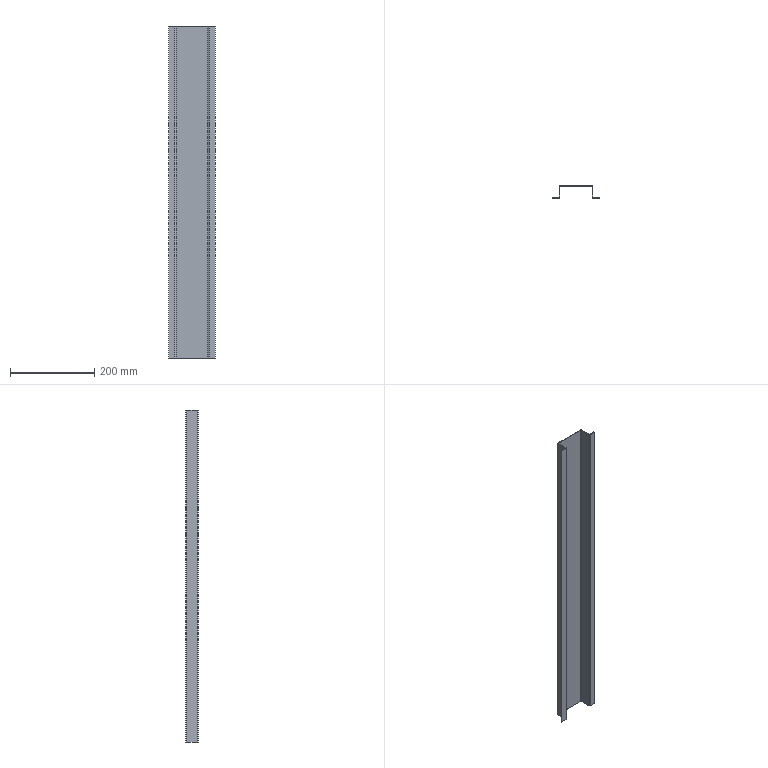Part | SolidWorks | features FlatPattern 1, SMBaseFlange 1, SheetMetal 1 | 1 solid | 38 faces | box 110 x 30 x 790 mm | volume 195352 mm3 | plane 30 | cylinder 8 | commonest cylinder face diameters 1 x4 4 x4
STEP:
#1=CARTESIAN_POINT('',(-40.,0.5,395.));
#2=VERTEX_POINT('',#1);
#3=CARTESIAN_POINT('',(-38.5,0.5,395.));
#4=VERTEX_POINT('',#3);
#5=CARTESIAN_POINT('',(-40.,0.5,395.));
#6=DIRECTION('',(1.,0.,0.));
#7=VECTOR('',#6,1000.);
#8=LINE('',#5,#7);
#9=EDGE_CURVE('',#2,#4,#8,.T.);
#10=ORIENTED_EDGE('',*,*,#9,.F.);
#11=CARTESIAN_POINT('',(-40.5,0.,395.));
#12=VERTEX_POINT('',#11);
#13=CARTESIAN_POINT('',(-40.5,0.5,395.));
#14=DIRECTION('',(0.,0.,-1.));
#15=DIRECTION('',(-1.,0.,0.));
#16=AXIS2_PLACEMENT_3D('',#13,#14,#15);
#17=CIRCLE('',#16,0.5);
#18=EDGE_CURVE('',#2,#12,#17,.T.);
#19=ORIENTED_EDGE('',*,*,#18,.T.);
#20=CARTESIAN_POINT('',(-40.5,-1.5,395.));
#21=VERTEX_POINT('',#20);
#22=CARTESIAN_POINT('',(-40.5,-1.5,395.));
#23=DIRECTION('',(0.,1.,0.));
#24=VECTOR('',#23,1000.);
#25=LINE('',#22,#24);
#26=EDGE_CURVE('',#21,#12,#25,.T.);
#27=ORIENTED_EDGE('',*,*,#26,.F.);
#28=CARTESIAN_POINT('',(-40.5,0.5,395.));
#29=DIRECTION('',(0.,0.,-1.));
#30=DIRECTION('',(1.,0.,0.));
#31=AXIS2_PLACEMENT_3D('',#28,#29,#30);
#32=CIRCLE('',#31,2.);
#33=EDGE_CURVE('',#4,#21,#32,.T.);
#34=ORIENTED_EDGE('',*,*,#33,.F.);
#35=EDGE_LOOP('',(#10,#19,#27,#34));
#36=FACE_OUTER_BOUND('',#35,.T.);
#37=CARTESIAN_POINT('',(-40.,0.5,395.));
#38=DIRECTION('',(0.,0.,1.));
#39=DIRECTION('',(1.,0.,0.));
#40=AXIS2_PLACEMENT_3D('',#37,#38,#39);
#41=PLANE('',#40);
#42=ADVANCED_FACE('',(#36),#41,.T.);
#43=CARTESIAN_POINT('',(-40.,26.5,395.));
#44=VERTEX_POINT('',#43);
#45=CARTESIAN_POINT('',(-40.,0.,395.));
#46=DIRECTION('',(0.,-1.,0.));
#47=VECTOR('',#46,1000.);
#48=LINE('',#45,#47);
#49=EDGE_CURVE('',#44,#2,#48,.T.);
#50=ORIENTED_EDGE('',*,*,#49,.T.);
#51=ORIENTED_EDGE('',*,*,#9,.T.);
#52=CARTESIAN_POINT('',(-38.5,26.5,395.));
#53=VERTEX_POINT('',#52);
#54=CARTESIAN_POINT('',(-38.5,0.,395.));
#55=DIRECTION('',(0.,-1.,0.));
#56=VECTOR('',#55,1000.);
#57=LINE('',#54,#56);
#58=EDGE_CURVE('',#53,#4,#57,.T.);
#59=ORIENTED_EDGE('',*,*,#58,.F.);
#60=CARTESIAN_POINT('',(-38.5,26.5,395.));
#61=DIRECTION('',(-1.,0.,0.));
#62=VECTOR('',#61,1000.);
#63=LINE('',#60,#62);
#64=EDGE_CURVE('',#53,#44,#63,.T.);
#65=ORIENTED_EDGE('',*,*,#64,.T.);
#66=EDGE_LOOP('',(#50,#51,#59,#65));
#67=FACE_OUTER_BOUND('',#66,.T.);
#68=CARTESIAN_POINT('',(-40.5,-1.5,395.));
#69=DIRECTION('',(0.,0.,1.));
#70=DIRECTION('',(1.,0.,0.));
#71=AXIS2_PLACEMENT_3D('',#68,#69,#70);
#72=PLANE('',#71);
#73=ADVANCED_FACE('',(#67),#72,.T.);
#74=CARTESIAN_POINT('',(-40.5,0.,-395.));
#75=VERTEX_POINT('',#74);
#76=CARTESIAN_POINT('',(-40.5,-1.5,-395.));
#77=VERTEX_POINT('',#76);
#78=CARTESIAN_POINT('',(-40.5,0.,-395.));
#79=DIRECTION('',(0.,-1.,0.));
#80=VECTOR('',#79,1000.);
#81=LINE('',#78,#80);
#82=EDGE_CURVE('',#75,#77,#81,.T.);
#83=ORIENTED_EDGE('',*,*,#82,.F.);
#84=CARTESIAN_POINT('',(-40.,0.5,-395.));
#85=VERTEX_POINT('',#84);
#86=CARTESIAN_POINT('',(-40.5,0.5,-395.));
#87=DIRECTION('',(0.,0.,-1.));
#88=DIRECTION('',(-1.,0.,0.));
#89=AXIS2_PLACEMENT_3D('',#86,#87,#88);
#90=CIRCLE('',#89,0.5);
#91=EDGE_CURVE('',#85,#75,#90,.T.);
#92=ORIENTED_EDGE('',*,*,#91,.F.);
#93=CARTESIAN_POINT('',(-38.5,0.5,-395.));
#94=VERTEX_POINT('',#93);
#95=CARTESIAN_POINT('',(-38.5,0.5,-395.));
#96=DIRECTION('',(-1.,0.,0.));
#97=VECTOR('',#96,1000.);
#98=LINE('',#95,#97);
#99=EDGE_CURVE('',#94,#85,#98,.T.);
#100=ORIENTED_EDGE('',*,*,#99,.F.);
#101=CARTESIAN_POINT('',(-40.5,0.5,-395.));
#102=DIRECTION('',(0.,0.,-1.));
#103=DIRECTION('',(1.,0.,0.));
#104=AXIS2_PLACEMENT_3D('',#101,#102,#103);
#105=CIRCLE('',#104,2.);
#106=EDGE_CURVE('',#94,#77,#105,.T.);
#107=ORIENTED_EDGE('',*,*,#106,.T.);
#108=EDGE_LOOP('',(#83,#92,#100,#107));
#109=FACE_OUTER_BOUND('',#108,.T.);
#110=CARTESIAN_POINT('',(-40.5,0.,-395.));
#111=DIRECTION('',(0.,0.,-1.));
#112=DIRECTION('',(-1.,0.,0.));
#113=AXIS2_PLACEMENT_3D('',#110,#111,#112);
#114=PLANE('',#113);
#115=ADVANCED_FACE('',(#109),#114,.T.);
#116=CARTESIAN_POINT('',(-55.,0.,-395.));
#117=VERTEX_POINT('',#116);
#118=CARTESIAN_POINT('',(-55.,0.,-395.));
#119=DIRECTION('',(-1.,0.,0.));
#120=VECTOR('',#119,1000.);
#121=LINE('',#118,#120);
#122=EDGE_CURVE('',#75,#117,#121,.T.);
#123=ORIENTED_EDGE('',*,*,#122,.F.);
#124=ORIENTED_EDGE('',*,*,#82,.T.);
#125=CARTESIAN_POINT('',(-55.,-1.5,-395.));
#126=VERTEX_POINT('',#125);
#127=CARTESIAN_POINT('',(-55.,-1.5,-395.));
#128=DIRECTION('',(-1.,0.,0.));
#129=VECTOR('',#128,1000.);
#130=LINE('',#127,#129);
#131=EDGE_CURVE('',#77,#126,#130,.T.);
#132=ORIENTED_EDGE('',*,*,#131,.T.);
#133=CARTESIAN_POINT('',(-55.,-1.5,-395.));
#134=DIRECTION('',(0.,1.,0.));
#135=VECTOR('',#134,1000.);
#136=LINE('',#133,#135);
#137=EDGE_CURVE('',#126,#117,#136,.T.);
#138=ORIENTED_EDGE('',*,*,#137,.T.);
#139=EDGE_LOOP('',(#123,#124,#132,#138));
#140=FACE_OUTER_BOUND('',#139,.T.);
#141=CARTESIAN_POINT('',(-38.5,0.5,-395.));
#142=DIRECTION('',(0.,0.,-1.));
#143=DIRECTION('',(-1.,0.,0.));
#144=AXIS2_PLACEMENT_3D('',#141,#142,#143);
#145=PLANE('',#144);
#146=ADVANCED_FACE('',(#140),#145,.T.);
#147=CARTESIAN_POINT('',(-38.,28.5,395.));
#148=VERTEX_POINT('',#147);
#149=CARTESIAN_POINT('',(-38.,27.,395.));
#150=VERTEX_POINT('',#149);
#151=CARTESIAN_POINT('',(-38.,28.5,395.));
#152=DIRECTION('',(0.,-1.,0.));
#153=VECTOR('',#152,1000.);
#154=LINE('',#151,#153);
#155=EDGE_CURVE('',#148,#150,#154,.T.);
#156=ORIENTED_EDGE('',*,*,#155,.F.);
#157=CARTESIAN_POINT('',(-38.,26.5,395.));
#158=DIRECTION('',(0.,0.,1.));
#159=DIRECTION('',(1.,0.,0.));
#160=AXIS2_PLACEMENT_3D('',#157,#158,#159);
#161=CIRCLE('',#160,2.);
#162=EDGE_CURVE('',#148,#44,#161,.T.);
#163=ORIENTED_EDGE('',*,*,#162,.T.);
#164=ORIENTED_EDGE('',*,*,#64,.F.);
#165=CARTESIAN_POINT('',(-38.,26.5,395.));
#166=DIRECTION('',(0.,0.,1.));
#167=DIRECTION('',(1.,0.,0.));
#168=AXIS2_PLACEMENT_3D('',#165,#166,#167);
#169=CIRCLE('',#168,0.5);
#170=EDGE_CURVE('',#150,#53,#169,.T.);
#171=ORIENTED_EDGE('',*,*,#170,.F.);
#172=EDGE_LOOP('',(#156,#163,#164,#171));
#173=FACE_OUTER_BOUND('',#172,.T.);
#174=CARTESIAN_POINT('',(-38.,28.5,395.));
#175=DIRECTION('',(0.,0.,1.));
#176=DIRECTION('',(1.,0.,0.));
#177=AXIS2_PLACEMENT_3D('',#174,#175,#176);
#178=PLANE('',#177);
#179=ADVANCED_FACE('',(#173),#178,.T.);
#180=CARTESIAN_POINT('',(38.,28.5,395.));
#181=VERTEX_POINT('',#180);
#182=CARTESIAN_POINT('',(-40.,28.5,395.));
#183=DIRECTION('',(-1.,0.,0.));
#184=VECTOR('',#183,1000.);
#185=LINE('',#182,#184);
#186=EDGE_CURVE('',#181,#148,#185,.T.);
#187=ORIENTED_EDGE('',*,*,#186,.T.);
#188=ORIENTED_EDGE('',*,*,#155,.T.);
#189=CARTESIAN_POINT('',(38.,27.,395.));
#190=VERTEX_POINT('',#189);
#191=CARTESIAN_POINT('',(-40.,27.,395.));
#192=DIRECTION('',(-1.,0.,0.));
#193=VECTOR('',#192,1000.);
#194=LINE('',#191,#193);
#195=EDGE_CURVE('',#190,#150,#194,.T.);
#196=ORIENTED_EDGE('',*,*,#195,.F.);
#197=CARTESIAN_POINT('',(38.,27.,395.));
#198=DIRECTION('',(0.,1.,0.));
#199=VECTOR('',#198,1000.);
#200=LINE('',#197,#199);
#201=EDGE_CURVE('',#190,#181,#200,.T.);
#202=ORIENTED_EDGE('',*,*,#201,.T.);
#203=EDGE_LOOP('',(#187,#188,#196,#202));
#204=FACE_OUTER_BOUND('',#203,.T.);
#205=CARTESIAN_POINT('',(-38.5,26.5,395.));
#206=DIRECTION('',(0.,0.,1.));
#207=DIRECTION('',(1.,0.,0.));
#208=AXIS2_PLACEMENT_3D('',#205,#206,#207);
#209=PLANE('',#208);
#210=ADVANCED_FACE('',(#204),#209,.T.);
#211=CARTESIAN_POINT('',(-40.,26.5,-395.));
#212=VERTEX_POINT('',#211);
#213=CARTESIAN_POINT('',(-38.5,26.5,-395.));
#214=VERTEX_POINT('',#213);
#215=CARTESIAN_POINT('',(-40.,26.5,-395.));
#216=DIRECTION('',(1.,0.,0.));
#217=VECTOR('',#216,1000.);
#218=LINE('',#215,#217);
#219=EDGE_CURVE('',#212,#214,#218,.T.);
#220=ORIENTED_EDGE('',*,*,#219,.F.);
#221=CARTESIAN_POINT('',(-38.,28.5,-395.));
#222=VERTEX_POINT('',#221);
#223=CARTESIAN_POINT('',(-38.,26.5,-395.));
#224=DIRECTION('',(0.,0.,1.));
#225=DIRECTION('',(1.,0.,0.));
#226=AXIS2_PLACEMENT_3D('',#223,#224,#225);
#227=CIRCLE('',#226,2.);
#228=EDGE_CURVE('',#222,#212,#227,.T.);
#229=ORIENTED_EDGE('',*,*,#228,.F.);
#230=CARTESIAN_POINT('',(-38.,27.,-395.));
#231=VERTEX_POINT('',#230);
#232=CARTESIAN_POINT('',(-38.,27.,-395.));
#233=DIRECTION('',(0.,1.,0.));
#234=VECTOR('',#233,1000.);
#235=LINE('',#232,#234);
#236=EDGE_CURVE('',#231,#222,#235,.T.);
#237=ORIENTED_EDGE('',*,*,#236,.F.);
#238=CARTESIAN_POINT('',(-38.,26.5,-395.));
#239=DIRECTION('',(0.,0.,1.));
#240=DIRECTION('',(1.,0.,0.));
#241=AXIS2_PLACEMENT_3D('',#238,#239,#240);
#242=CIRCLE('',#241,0.5);
#243=EDGE_CURVE('',#231,#214,#242,.T.);
#244=ORIENTED_EDGE('',*,*,#243,.T.);
#245=EDGE_LOOP('',(#220,#229,#237,#244));
#246=FACE_OUTER_BOUND('',#245,.T.);
#247=CARTESIAN_POINT('',(-40.,26.5,-395.));
#248=DIRECTION('',(0.,0.,-1.));
#249=DIRECTION('',(-1.,0.,0.));
#250=AXIS2_PLACEMENT_3D('',#247,#248,#249);
#251=PLANE('',#250);
#252=ADVANCED_FACE('',(#246),#251,.T.);
#253=CARTESIAN_POINT('',(-40.,0.,-395.));
#254=DIRECTION('',(0.,-1.,0.));
#255=VECTOR('',#254,1000.);
#256=LINE('',#253,#255);
#257=EDGE_CURVE('',#212,#85,#256,.T.);
#258=ORIENTED_EDGE('',*,*,#257,.F.);
#259=ORIENTED_EDGE('',*,*,#219,.T.);
#260=CARTESIAN_POINT('',(-38.5,0.,-395.));
#261=DIRECTION('',(0.,-1.,0.));
#262=VECTOR('',#261,1000.);
#263=LINE('',#260,#262);
#264=EDGE_CURVE('',#214,#94,#263,.T.);
#265=ORIENTED_EDGE('',*,*,#264,.T.);
#266=ORIENTED_EDGE('',*,*,#99,.T.);
#267=EDGE_LOOP('',(#258,#259,#265,#266));
#268=FACE_OUTER_BOUND('',#267,.T.);
#269=CARTESIAN_POINT('',(-38.,27.,-395.));
#270=DIRECTION('',(0.,0.,-1.));
#271=DIRECTION('',(-1.,0.,0.));
#272=AXIS2_PLACEMENT_3D('',#269,#270,#271);
#273=PLANE('',#272);
#274=ADVANCED_FACE('',(#268),#273,.T.);
#275=CARTESIAN_POINT('',(40.,26.5,395.));
#276=VERTEX_POINT('',#275);
#277=CARTESIAN_POINT('',(38.5,26.5,395.));
#278=VERTEX_POINT('',#277);
#279=CARTESIAN_POINT('',(40.,26.5,395.));
#280=DIRECTION('',(-1.,0.,0.));
#281=VECTOR('',#280,1000.);
#282=LINE('',#279,#281);
#283=EDGE_CURVE('',#276,#278,#282,.T.);
#284=ORIENTED_EDGE('',*,*,#283,.F.);
#285=CARTESIAN_POINT('',(38.,26.5,395.));
#286=DIRECTION('',(0.,0.,1.));
#287=DIRECTION('',(1.,0.,0.));
#288=AXIS2_PLACEMENT_3D('',#285,#286,#287);
#289=CIRCLE('',#288,2.);
#290=EDGE_CURVE('',#276,#181,#289,.T.);
#291=ORIENTED_EDGE('',*,*,#290,.T.);
#292=ORIENTED_EDGE('',*,*,#201,.F.);
#293=CARTESIAN_POINT('',(38.,26.5,395.));
#294=DIRECTION('',(0.,0.,1.));
#295=DIRECTION('',(1.,0.,0.));
#296=AXIS2_PLACEMENT_3D('',#293,#294,#295);
#297=CIRCLE('',#296,0.5);
#298=EDGE_CURVE('',#278,#190,#297,.T.);
#299=ORIENTED_EDGE('',*,*,#298,.F.);
#300=EDGE_LOOP('',(#284,#291,#292,#299));
#301=FACE_OUTER_BOUND('',#300,.T.);
#302=CARTESIAN_POINT('',(40.,26.5,395.));
#303=DIRECTION('',(0.,0.,1.));
#304=DIRECTION('',(1.,0.,0.));
#305=AXIS2_PLACEMENT_3D('',#302,#303,#304);
#306=PLANE('',#305);
#307=ADVANCED_FACE('',(#301),#306,.T.);
#308=CARTESIAN_POINT('',(40.,0.5,395.));
#309=VERTEX_POINT('',#308);
#310=CARTESIAN_POINT('',(40.,0.,395.));
#311=DIRECTION('',(0.,1.,0.));
#312=VECTOR('',#311,1000.);
#313=LINE('',#310,#312);
#314=EDGE_CURVE('',#309,#276,#313,.T.);
#315=ORIENTED_EDGE('',*,*,#314,.T.);
#316=ORIENTED_EDGE('',*,*,#283,.T.);
#317=CARTESIAN_POINT('',(38.5,0.5,395.));
#318=VERTEX_POINT('',#317);
#319=CARTESIAN_POINT('',(38.5,0.,395.));
#320=DIRECTION('',(0.,1.,0.));
#321=VECTOR('',#320,1000.);
#322=LINE('',#319,#321);
#323=EDGE_CURVE('',#318,#278,#322,.T.);
#324=ORIENTED_EDGE('',*,*,#323,.F.);
#325=CARTESIAN_POINT('',(38.5,0.5,395.));
#326=DIRECTION('',(1.,0.,0.));
#327=VECTOR('',#326,1000.);
#328=LINE('',#325,#327);
#329=EDGE_CURVE('',#318,#309,#328,.T.);
#330=ORIENTED_EDGE('',*,*,#329,.T.);
#331=EDGE_LOOP('',(#315,#316,#324,#330));
#332=FACE_OUTER_BOUND('',#331,.T.);
#333=CARTESIAN_POINT('',(38.,27.,395.));
#334=DIRECTION('',(0.,0.,1.));
#335=DIRECTION('',(1.,0.,0.));
#336=AXIS2_PLACEMENT_3D('',#333,#334,#335);
#337=PLANE('',#336);
#338=ADVANCED_FACE('',(#332),#337,.T.);
#339=CARTESIAN_POINT('',(38.,28.5,-395.));
#340=VERTEX_POINT('',#339);
#341=CARTESIAN_POINT('',(38.,27.,-395.));
#342=VERTEX_POINT('',#341);
#343=CARTESIAN_POINT('',(38.,28.5,-395.));
#344=DIRECTION('',(0.,-1.,0.));
#345=VECTOR('',#344,1000.);
#346=LINE('',#343,#345);
#347=EDGE_CURVE('',#340,#342,#346,.T.);
#348=ORIENTED_EDGE('',*,*,#347,.F.);
#349=CARTESIAN_POINT('',(40.,26.5,-395.));
#350=VERTEX_POINT('',#349);
#351=CARTESIAN_POINT('',(38.,26.5,-395.));
#352=DIRECTION('',(0.,0.,1.));
#353=DIRECTION('',(1.,0.,0.));
#354=AXIS2_PLACEMENT_3D('',#351,#352,#353);
#355=CIRCLE('',#354,2.);
#356=EDGE_CURVE('',#350,#340,#355,.T.);
#357=ORIENTED_EDGE('',*,*,#356,.F.);
#358=CARTESIAN_POINT('',(38.5,26.5,-395.));
#359=VERTEX_POINT('',#358);
#360=CARTESIAN_POINT('',(38.5,26.5,-395.));
#361=DIRECTION('',(1.,0.,0.));
#362=VECTOR('',#361,1000.);
#363=LINE('',#360,#362);
#364=EDGE_CURVE('',#359,#350,#363,.T.);
#365=ORIENTED_EDGE('',*,*,#364,.F.);
#366=CARTESIAN_POINT('',(38.,26.5,-395.));
#367=DIRECTION('',(0.,0.,1.));
#368=DIRECTION('',(1.,0.,0.));
#369=AXIS2_PLACEMENT_3D('',#366,#367,#368);
#370=CIRCLE('',#369,0.5);
#371=EDGE_CURVE('',#359,#342,#370,.T.);
#372=ORIENTED_EDGE('',*,*,#371,.T.);
#373=EDGE_LOOP('',(#348,#357,#365,#372));
#374=FACE_OUTER_BOUND('',#373,.T.);
#375=CARTESIAN_POINT('',(38.,28.5,-395.));
#376=DIRECTION('',(0.,0.,-1.));
#377=DIRECTION('',(-1.,0.,0.));
#378=AXIS2_PLACEMENT_3D('',#375,#376,#377);
#379=PLANE('',#378);
#380=ADVANCED_FACE('',(#374),#379,.T.);
#381=CARTESIAN_POINT('',(-40.,28.5,-395.));
#382=DIRECTION('',(-1.,0.,0.));
#383=VECTOR('',#382,1000.);
#384=LINE('',#381,#383);
#385=EDGE_CURVE('',#340,#222,#384,.T.);
#386=ORIENTED_EDGE('',*,*,#385,.F.);
#387=ORIENTED_EDGE('',*,*,#347,.T.);
#388=CARTESIAN_POINT('',(-40.,27.,-395.));
#389=DIRECTION('',(-1.,0.,0.));
#390=VECTOR('',#389,1000.);
#391=LINE('',#388,#390);
#392=EDGE_CURVE('',#342,#231,#391,.T.);
#393=ORIENTED_EDGE('',*,*,#392,.T.);
#394=ORIENTED_EDGE('',*,*,#236,.T.);
#395=EDGE_LOOP('',(#386,#387,#393,#394));
#396=FACE_OUTER_BOUND('',#395,.T.);
#397=CARTESIAN_POINT('',(38.5,26.5,-395.));
#398=DIRECTION('',(0.,0.,-1.));
#399=DIRECTION('',(-1.,0.,0.));
#400=AXIS2_PLACEMENT_3D('',#397,#398,#399);
#401=PLANE('',#400);
#402=ADVANCED_FACE('',(#396),#401,.T.);
#403=CARTESIAN_POINT('',(40.5,0.,395.));
#404=VERTEX_POINT('',#403);
#405=CARTESIAN_POINT('',(40.5,-1.5,395.));
#406=VERTEX_POINT('',#405);
#407=CARTESIAN_POINT('',(40.5,0.,395.));
#408=DIRECTION('',(0.,-1.,0.));
#409=VECTOR('',#408,1000.);
#410=LINE('',#407,#409);
#411=EDGE_CURVE('',#404,#406,#410,.T.);
#412=ORIENTED_EDGE('',*,*,#411,.F.);
#413=CARTESIAN_POINT('',(40.5,0.5,395.));
#414=DIRECTION('',(0.,0.,-1.));
#415=DIRECTION('',(-1.,0.,0.));
#416=AXIS2_PLACEMENT_3D('',#413,#414,#415);
#417=CIRCLE('',#416,0.5);
#418=EDGE_CURVE('',#404,#309,#417,.T.);
#419=ORIENTED_EDGE('',*,*,#418,.T.);
#420=ORIENTED_EDGE('',*,*,#329,.F.);
#421=CARTESIAN_POINT('',(40.5,0.5,395.));
#422=DIRECTION('',(0.,0.,-1.));
#423=DIRECTION('',(1.,0.,0.));
#424=AXIS2_PLACEMENT_3D('',#421,#422,#423);
#425=CIRCLE('',#424,2.);
#426=EDGE_CURVE('',#406,#318,#425,.T.);
#427=ORIENTED_EDGE('',*,*,#426,.F.);
#428=EDGE_LOOP('',(#412,#419,#420,#427));
#429=FACE_OUTER_BOUND('',#428,.T.);
#430=CARTESIAN_POINT('',(40.5,0.,395.));
#431=DIRECTION('',(0.,0.,1.));
#432=DIRECTION('',(1.,0.,0.));
#433=AXIS2_PLACEMENT_3D('',#430,#431,#432);
#434=PLANE('',#433);
#435=ADVANCED_FACE('',(#429),#434,.T.);
#436=CARTESIAN_POINT('',(55.,0.,395.));
#437=VERTEX_POINT('',#436);
#438=CARTESIAN_POINT('',(55.,0.,395.));
#439=DIRECTION('',(-1.,0.,0.));
#440=VECTOR('',#439,1000.);
#441=LINE('',#438,#440);
#442=EDGE_CURVE('',#437,#404,#441,.T.);
#443=ORIENTED_EDGE('',*,*,#442,.T.);
#444=ORIENTED_EDGE('',*,*,#411,.T.);
#445=CARTESIAN_POINT('',(55.,-1.5,395.));
#446=VERTEX_POINT('',#445);
#447=CARTESIAN_POINT('',(55.,-1.5,395.));
#448=DIRECTION('',(-1.,0.,0.));
#449=VECTOR('',#448,1000.);
#450=LINE('',#447,#449);
#451=EDGE_CURVE('',#446,#406,#450,.T.);
#452=ORIENTED_EDGE('',*,*,#451,.F.);
#453=CARTESIAN_POINT('',(55.,0.,395.));
#454=DIRECTION('',(0.,-1.,0.));
#455=VECTOR('',#454,1000.);
#456=LINE('',#453,#455);
#457=EDGE_CURVE('',#437,#446,#456,.T.);
#458=ORIENTED_EDGE('',*,*,#457,.F.);
#459=EDGE_LOOP('',(#443,#444,#452,#458));
#460=FACE_OUTER_BOUND('',#459,.T.);
#461=CARTESIAN_POINT('',(38.5,0.5,395.));
#462=DIRECTION('',(0.,0.,1.));
#463=DIRECTION('',(1.,0.,0.));
#464=AXIS2_PLACEMENT_3D('',#461,#462,#463);
#465=PLANE('',#464);
#466=ADVANCED_FACE('',(#460),#465,.T.);
#467=CARTESIAN_POINT('',(40.,0.5,-395.));
#468=VERTEX_POINT('',#467);
#469=CARTESIAN_POINT('',(38.5,0.5,-395.));
#470=VERTEX_POINT('',#469);
#471=CARTESIAN_POINT('',(40.,0.5,-395.));
#472=DIRECTION('',(-1.,0.,0.));
#473=VECTOR('',#472,1000.);
#474=LINE('',#471,#473);
#475=EDGE_CURVE('',#468,#470,#474,.T.);
#476=ORIENTED_EDGE('',*,*,#475,.F.);
#477=CARTESIAN_POINT('',(40.5,0.,-395.));
#478=VERTEX_POINT('',#477);
#479=CARTESIAN_POINT('',(40.5,0.5,-395.));
#480=DIRECTION('',(0.,0.,-1.));
#481=DIRECTION('',(-1.,0.,0.));
#482=AXIS2_PLACEMENT_3D('',#479,#480,#481);
#483=CIRCLE('',#482,0.5);
#484=EDGE_CURVE('',#478,#468,#483,.T.);
#485=ORIENTED_EDGE('',*,*,#484,.F.);
#486=CARTESIAN_POINT('',(40.5,-1.5,-395.));
#487=VERTEX_POINT('',#486);
#488=CARTESIAN_POINT('',(40.5,-1.5,-395.));
#489=DIRECTION('',(0.,1.,0.));
#490=VECTOR('',#489,1000.);
#491=LINE('',#488,#490);
#492=EDGE_CURVE('',#487,#478,#491,.T.);
#493=ORIENTED_EDGE('',*,*,#492,.F.);
#494=CARTESIAN_POINT('',(40.5,0.5,-395.));
#495=DIRECTION('',(0.,0.,-1.));
#496=DIRECTION('',(1.,0.,0.));
#497=AXIS2_PLACEMENT_3D('',#494,#495,#496);
#498=CIRCLE('',#497,2.);
#499=EDGE_CURVE('',#487,#470,#498,.T.);
#500=ORIENTED_EDGE('',*,*,#499,.T.);
#501=EDGE_LOOP('',(#476,#485,#493,#500));
#502=FACE_OUTER_BOUND('',#501,.T.);
#503=CARTESIAN_POINT('',(40.,0.5,-395.));
#504=DIRECTION('',(0.,0.,-1.));
#505=DIRECTION('',(-1.,0.,0.));
#506=AXIS2_PLACEMENT_3D('',#503,#504,#505);
#507=PLANE('',#506);
#508=ADVANCED_FACE('',(#502),#507,.T.);
#509=CARTESIAN_POINT('',(40.,0.,-395.));
#510=DIRECTION('',(0.,1.,0.));
#511=VECTOR('',#510,1000.);
#512=LINE('',#509,#511);
#513=EDGE_CURVE('',#468,#350,#512,.T.);
#514=ORIENTED_EDGE('',*,*,#513,.F.);
#515=ORIENTED_EDGE('',*,*,#475,.T.);
#516=CARTESIAN_POINT('',(38.5,0.,-395.));
#517=DIRECTION('',(0.,1.,0.));
#518=VECTOR('',#517,1000.);
#519=LINE('',#516,#518);
#520=EDGE_CURVE('',#470,#359,#519,.T.);
#521=ORIENTED_EDGE('',*,*,#520,.T.);
#522=ORIENTED_EDGE('',*,*,#364,.T.);
#523=EDGE_LOOP('',(#514,#515,#521,#522));
#524=FACE_OUTER_BOUND('',#523,.T.);
#525=CARTESIAN_POINT('',(40.5,-1.5,-395.));
#526=DIRECTION('',(0.,0.,-1.));
#527=DIRECTION('',(-1.,0.,0.));
#528=AXIS2_PLACEMENT_3D('',#525,#526,#527);
#529=PLANE('',#528);
#530=ADVANCED_FACE('',(#524),#529,.T.);
#531=ORIENTED_EDGE('',*,*,#122,.T.);
#532=CARTESIAN_POINT('',(-55.,0.,395.));
#533=VERTEX_POINT('',#532);
#534=CARTESIAN_POINT('',(-55.,0.,395.));
#535=DIRECTION('',(0.,0.,-1.));
#536=VECTOR('',#535,1000.);
#537=LINE('',#534,#536);
#538=EDGE_CURVE('',#533,#117,#537,.T.);
#539=ORIENTED_EDGE('',*,*,#538,.F.);
#540=CARTESIAN_POINT('',(-55.,0.,395.));
#541=DIRECTION('',(-1.,0.,0.));
#542=VECTOR('',#541,1000.);
#543=LINE('',#540,#542);
#544=EDGE_CURVE('',#12,#533,#543,.T.);
#545=ORIENTED_EDGE('',*,*,#544,.F.);
#546=CARTESIAN_POINT('',(-40.5,0.,395.));
#547=DIRECTION('',(0.,0.,-1.));
#548=VECTOR('',#547,1000.);
#549=LINE('',#546,#548);
#550=EDGE_CURVE('',#12,#75,#549,.T.);
#551=ORIENTED_EDGE('',*,*,#550,.T.);
#552=EDGE_LOOP('',(#531,#539,#545,#551));
#553=FACE_OUTER_BOUND('',#552,.T.);
#554=CARTESIAN_POINT('',(-55.,0.,395.));
#555=DIRECTION('',(0.,-1.,0.));
#556=DIRECTION('',(0.,0.,-1.));
#557=AXIS2_PLACEMENT_3D('',#554,#555,#556);
#558=PLANE('',#557);
#559=ADVANCED_FACE('',(#553),#558,.F.);
#560=ORIENTED_EDGE('',*,*,#137,.F.);
#561=CARTESIAN_POINT('',(-55.,-1.5,395.));
#562=VERTEX_POINT('',#561);
#563=CARTESIAN_POINT('',(-55.,-1.5,395.));
#564=DIRECTION('',(0.,0.,-1.));
#565=VECTOR('',#564,1000.);
#566=LINE('',#563,#565);
#567=EDGE_CURVE('',#562,#126,#566,.T.);
#568=ORIENTED_EDGE('',*,*,#567,.F.);
#569=CARTESIAN_POINT('',(-55.,-1.5,395.));
#570=DIRECTION('',(0.,1.,0.));
#571=VECTOR('',#570,1000.);
#572=LINE('',#569,#571);
#573=EDGE_CURVE('',#562,#533,#572,.T.);
#574=ORIENTED_EDGE('',*,*,#573,.T.);
#575=ORIENTED_EDGE('',*,*,#538,.T.);
#576=EDGE_LOOP('',(#560,#568,#574,#575));
#577=FACE_OUTER_BOUND('',#576,.T.);
#578=CARTESIAN_POINT('',(-55.,-1.5,395.));
#579=DIRECTION('',(-1.,0.,0.));
#580=DIRECTION('',(0.,0.,1.));
#581=AXIS2_PLACEMENT_3D('',#578,#579,#580);
#582=PLANE('',#581);
#583=ADVANCED_FACE('',(#577),#582,.T.);
#584=ORIENTED_EDGE('',*,*,#131,.F.);
#585=CARTESIAN_POINT('',(-40.5,-1.5,395.));
#586=DIRECTION('',(0.,0.,-1.));
#587=VECTOR('',#586,1000.);
#588=LINE('',#585,#587);
#589=EDGE_CURVE('',#21,#77,#588,.T.);
#590=ORIENTED_EDGE('',*,*,#589,.F.);
#591=CARTESIAN_POINT('',(-55.,-1.5,395.));
#592=DIRECTION('',(-1.,0.,0.));
#593=VECTOR('',#592,1000.);
#594=LINE('',#591,#593);
#595=EDGE_CURVE('',#21,#562,#594,.T.);
#596=ORIENTED_EDGE('',*,*,#595,.T.);
#597=ORIENTED_EDGE('',*,*,#567,.T.);
#598=EDGE_LOOP('',(#584,#590,#596,#597));
#599=FACE_OUTER_BOUND('',#598,.T.);
#600=CARTESIAN_POINT('',(-55.,-1.5,395.));
#601=DIRECTION('',(0.,-1.,0.));
#602=DIRECTION('',(0.,0.,-1.));
#603=AXIS2_PLACEMENT_3D('',#600,#601,#602);
#604=PLANE('',#603);
#605=ADVANCED_FACE('',(#599),#604,.T.);
#606=ORIENTED_EDGE('',*,*,#106,.F.);
#607=CARTESIAN_POINT('',(-38.5,0.5,395.));
#608=DIRECTION('',(0.,0.,-1.));
#609=VECTOR('',#608,1000.);
#610=LINE('',#607,#609);
#611=EDGE_CURVE('',#4,#94,#610,.T.);
#612=ORIENTED_EDGE('',*,*,#611,.F.);
#613=ORIENTED_EDGE('',*,*,#33,.T.);
#614=ORIENTED_EDGE('',*,*,#589,.T.);
#615=EDGE_LOOP('',(#606,#612,#613,#614));
#616=FACE_OUTER_BOUND('',#615,.T.);
#617=CARTESIAN_POINT('',(-40.5,0.5,395.));
#618=DIRECTION('',(0.,0.,-1.));
#619=DIRECTION('',(-1.,0.,0.));
#620=AXIS2_PLACEMENT_3D('',#617,#618,#619);
#621=CYLINDRICAL_SURFACE('',#620,2.);
#622=ADVANCED_FACE('',(#616),#621,.T.);
#623=ORIENTED_EDGE('',*,*,#264,.F.);
#624=CARTESIAN_POINT('',(-38.5,26.5,395.));
#625=DIRECTION('',(0.,0.,-1.));
#626=VECTOR('',#625,1000.);
#627=LINE('',#624,#626);
#628=EDGE_CURVE('',#53,#214,#627,.T.);
#629=ORIENTED_EDGE('',*,*,#628,.F.);
#630=ORIENTED_EDGE('',*,*,#58,.T.);
#631=ORIENTED_EDGE('',*,*,#611,.T.);
#632=EDGE_LOOP('',(#623,#629,#630,#631));
#633=FACE_OUTER_BOUND('',#632,.T.);
#634=CARTESIAN_POINT('',(-38.5,0.,395.));
#635=DIRECTION('',(1.,0.,0.));
#636=DIRECTION('',(0.,1.,0.));
#637=AXIS2_PLACEMENT_3D('',#634,#635,#636);
#638=PLANE('',#637);
#639=ADVANCED_FACE('',(#633),#638,.T.);
#640=ORIENTED_EDGE('',*,*,#243,.F.);
#641=CARTESIAN_POINT('',(-38.,27.,395.));
#642=DIRECTION('',(0.,0.,-1.));
#643=VECTOR('',#642,1000.);
#644=LINE('',#641,#643);
#645=EDGE_CURVE('',#150,#231,#644,.T.);
#646=ORIENTED_EDGE('',*,*,#645,.F.);
#647=ORIENTED_EDGE('',*,*,#170,.T.);
#648=ORIENTED_EDGE('',*,*,#628,.T.);
#649=EDGE_LOOP('',(#640,#646,#647,#648));
#650=FACE_OUTER_BOUND('',#649,.T.);
#651=CARTESIAN_POINT('',(-38.,26.5,395.));
#652=DIRECTION('',(0.,0.,-1.));
#653=DIRECTION('',(-1.,0.,0.));
#654=AXIS2_PLACEMENT_3D('',#651,#652,#653);
#655=CYLINDRICAL_SURFACE('',#654,0.5);
#656=ADVANCED_FACE('',(#650),#655,.F.);
#657=ORIENTED_EDGE('',*,*,#392,.F.);
#658=CARTESIAN_POINT('',(38.,27.,395.));
#659=DIRECTION('',(0.,0.,-1.));
#660=VECTOR('',#659,1000.);
#661=LINE('',#658,#660);
#662=EDGE_CURVE('',#190,#342,#661,.T.);
#663=ORIENTED_EDGE('',*,*,#662,.F.);
#664=ORIENTED_EDGE('',*,*,#195,.T.);
#665=ORIENTED_EDGE('',*,*,#645,.T.);
#666=EDGE_LOOP('',(#657,#663,#664,#665));
#667=FACE_OUTER_BOUND('',#666,.T.);
#668=CARTESIAN_POINT('',(-40.,27.,395.));
#669=DIRECTION('',(0.,-1.,0.));
#670=DIRECTION('',(0.,0.,-1.));
#671=AXIS2_PLACEMENT_3D('',#668,#669,#670);
#672=PLANE('',#671);
#673=ADVANCED_FACE('',(#667),#672,.T.);
#674=ORIENTED_EDGE('',*,*,#371,.F.);
#675=CARTESIAN_POINT('',(38.5,26.5,395.));
#676=DIRECTION('',(0.,0.,-1.));
#677=VECTOR('',#676,1000.);
#678=LINE('',#675,#677);
#679=EDGE_CURVE('',#278,#359,#678,.T.);
#680=ORIENTED_EDGE('',*,*,#679,.F.);
#681=ORIENTED_EDGE('',*,*,#298,.T.);
#682=ORIENTED_EDGE('',*,*,#662,.T.);
#683=EDGE_LOOP('',(#674,#680,#681,#682));
#684=FACE_OUTER_BOUND('',#683,.T.);
#685=CARTESIAN_POINT('',(38.,26.5,395.));
#686=DIRECTION('',(0.,0.,-1.));
#687=DIRECTION('',(-1.,0.,0.));
#688=AXIS2_PLACEMENT_3D('',#685,#686,#687);
#689=CYLINDRICAL_SURFACE('',#688,0.5);
#690=ADVANCED_FACE('',(#684),#689,.F.);
#691=ORIENTED_EDGE('',*,*,#520,.F.);
#692=CARTESIAN_POINT('',(38.5,0.5,395.));
#693=DIRECTION('',(0.,0.,-1.));
#694=VECTOR('',#693,1000.);
#695=LINE('',#692,#694);
#696=EDGE_CURVE('',#318,#470,#695,.T.);
#697=ORIENTED_EDGE('',*,*,#696,.F.);
#698=ORIENTED_EDGE('',*,*,#323,.T.);
#699=ORIENTED_EDGE('',*,*,#679,.T.);
#700=EDGE_LOOP('',(#691,#697,#698,#699));
#701=FACE_OUTER_BOUND('',#700,.T.);
#702=CARTESIAN_POINT('',(38.5,0.,395.));
#703=DIRECTION('',(-1.,0.,0.));
#704=DIRECTION('',(0.,-1.,0.));
#705=AXIS2_PLACEMENT_3D('',#702,#703,#704);
#706=PLANE('',#705);
#707=ADVANCED_FACE('',(#701),#706,.T.);
#708=ORIENTED_EDGE('',*,*,#499,.F.);
#709=CARTESIAN_POINT('',(40.5,-1.5,395.));
#710=DIRECTION('',(0.,0.,-1.));
#711=VECTOR('',#710,1000.);
#712=LINE('',#709,#711);
#713=EDGE_CURVE('',#406,#487,#712,.T.);
#714=ORIENTED_EDGE('',*,*,#713,.F.);
#715=ORIENTED_EDGE('',*,*,#426,.T.);
#716=ORIENTED_EDGE('',*,*,#696,.T.);
#717=EDGE_LOOP('',(#708,#714,#715,#716));
#718=FACE_OUTER_BOUND('',#717,.T.);
#719=CARTESIAN_POINT('',(40.5,0.5,395.));
#720=DIRECTION('',(0.,0.,-1.));
#721=DIRECTION('',(-1.,0.,0.));
#722=AXIS2_PLACEMENT_3D('',#719,#720,#721);
#723=CYLINDRICAL_SURFACE('',#722,2.);
#724=ADVANCED_FACE('',(#718),#723,.T.);
#725=CARTESIAN_POINT('',(55.,-1.5,-395.));
#726=VERTEX_POINT('',#725);
#727=CARTESIAN_POINT('',(55.,-1.5,-395.));
#728=DIRECTION('',(-1.,0.,0.));
#729=VECTOR('',#728,1000.);
#730=LINE('',#727,#729);
#731=EDGE_CURVE('',#726,#487,#730,.T.);
#732=ORIENTED_EDGE('',*,*,#731,.F.);
#733=CARTESIAN_POINT('',(55.,-1.5,395.));
#734=DIRECTION('',(0.,0.,-1.));
#735=VECTOR('',#734,1000.);
#736=LINE('',#733,#735);
#737=EDGE_CURVE('',#446,#726,#736,.T.);
#738=ORIENTED_EDGE('',*,*,#737,.F.);
#739=ORIENTED_EDGE('',*,*,#451,.T.);
#740=ORIENTED_EDGE('',*,*,#713,.T.);
#741=EDGE_LOOP('',(#732,#738,#739,#740));
#742=FACE_OUTER_BOUND('',#741,.T.);
#743=CARTESIAN_POINT('',(55.,-1.5,395.));
#744=DIRECTION('',(0.,-1.,0.));
#745=DIRECTION('',(0.,0.,-1.));
#746=AXIS2_PLACEMENT_3D('',#743,#744,#745);
#747=PLANE('',#746);
#748=ADVANCED_FACE('',(#742),#747,.T.);
#749=CARTESIAN_POINT('',(55.,0.,-395.));
#750=VERTEX_POINT('',#749);
#751=CARTESIAN_POINT('',(55.,0.,-395.));
#752=DIRECTION('',(0.,-1.,0.));
#753=VECTOR('',#752,1000.);
#754=LINE('',#751,#753);
#755=EDGE_CURVE('',#750,#726,#754,.T.);
#756=ORIENTED_EDGE('',*,*,#755,.F.);
#757=CARTESIAN_POINT('',(55.,0.,395.));
#758=DIRECTION('',(0.,0.,-1.));
#759=VECTOR('',#758,1000.);
#760=LINE('',#757,#759);
#761=EDGE_CURVE('',#437,#750,#760,.T.);
#762=ORIENTED_EDGE('',*,*,#761,.F.);
#763=ORIENTED_EDGE('',*,*,#457,.T.);
#764=ORIENTED_EDGE('',*,*,#737,.T.);
#765=EDGE_LOOP('',(#756,#762,#763,#764));
#766=FACE_OUTER_BOUND('',#765,.T.);
#767=CARTESIAN_POINT('',(55.,0.,395.));
#768=DIRECTION('',(1.,0.,0.));
#769=DIRECTION('',(0.,0.,-1.));
#770=AXIS2_PLACEMENT_3D('',#767,#768,#769);
#771=PLANE('',#770);
#772=ADVANCED_FACE('',(#766),#771,.T.);
#773=CARTESIAN_POINT('',(55.,0.,-395.));
#774=DIRECTION('',(-1.,0.,0.));
#775=VECTOR('',#774,1000.);
#776=LINE('',#773,#775);
#777=EDGE_CURVE('',#750,#478,#776,.T.);
#778=ORIENTED_EDGE('',*,*,#777,.T.);
#779=CARTESIAN_POINT('',(40.5,0.,395.));
#780=DIRECTION('',(0.,0.,-1.));
#781=VECTOR('',#780,1000.);
#782=LINE('',#779,#781);
#783=EDGE_CURVE('',#404,#478,#782,.T.);
#784=ORIENTED_EDGE('',*,*,#783,.F.);
#785=ORIENTED_EDGE('',*,*,#442,.F.);
#786=ORIENTED_EDGE('',*,*,#761,.T.);
#787=EDGE_LOOP('',(#778,#784,#785,#786));
#788=FACE_OUTER_BOUND('',#787,.T.);
#789=CARTESIAN_POINT('',(55.,0.,395.));
#790=DIRECTION('',(0.,-1.,0.));
#791=DIRECTION('',(0.,0.,-1.));
#792=AXIS2_PLACEMENT_3D('',#789,#790,#791);
#793=PLANE('',#792);
#794=ADVANCED_FACE('',(#788),#793,.F.);
#795=ORIENTED_EDGE('',*,*,#484,.T.);
#796=CARTESIAN_POINT('',(40.,0.5,395.));
#797=DIRECTION('',(0.,0.,-1.));
#798=VECTOR('',#797,1000.);
#799=LINE('',#796,#798);
#800=EDGE_CURVE('',#309,#468,#799,.T.);
#801=ORIENTED_EDGE('',*,*,#800,.F.);
#802=ORIENTED_EDGE('',*,*,#418,.F.);
#803=ORIENTED_EDGE('',*,*,#783,.T.);
#804=EDGE_LOOP('',(#795,#801,#802,#803));
#805=FACE_OUTER_BOUND('',#804,.T.);
#806=CARTESIAN_POINT('',(40.5,0.5,395.));
#807=DIRECTION('',(0.,0.,-1.));
#808=DIRECTION('',(-1.,0.,0.));
#809=AXIS2_PLACEMENT_3D('',#806,#807,#808);
#810=CYLINDRICAL_SURFACE('',#809,0.5);
#811=ADVANCED_FACE('',(#805),#810,.F.);
#812=ORIENTED_EDGE('',*,*,#513,.T.);
#813=CARTESIAN_POINT('',(40.,26.5,395.));
#814=DIRECTION('',(0.,0.,-1.));
#815=VECTOR('',#814,1000.);
#816=LINE('',#813,#815);
#817=EDGE_CURVE('',#276,#350,#816,.T.);
#818=ORIENTED_EDGE('',*,*,#817,.F.);
#819=ORIENTED_EDGE('',*,*,#314,.F.);
#820=ORIENTED_EDGE('',*,*,#800,.T.);
#821=EDGE_LOOP('',(#812,#818,#819,#820));
#822=FACE_OUTER_BOUND('',#821,.T.);
#823=CARTESIAN_POINT('',(40.,0.,395.));
#824=DIRECTION('',(-1.,0.,0.));
#825=DIRECTION('',(0.,-1.,0.));
#826=AXIS2_PLACEMENT_3D('',#823,#824,#825);
#827=PLANE('',#826);
#828=ADVANCED_FACE('',(#822),#827,.F.);
#829=ORIENTED_EDGE('',*,*,#356,.T.);
#830=CARTESIAN_POINT('',(38.,28.5,395.));
#831=DIRECTION('',(0.,0.,-1.));
#832=VECTOR('',#831,1000.);
#833=LINE('',#830,#832);
#834=EDGE_CURVE('',#181,#340,#833,.T.);
#835=ORIENTED_EDGE('',*,*,#834,.F.);
#836=ORIENTED_EDGE('',*,*,#290,.F.);
#837=ORIENTED_EDGE('',*,*,#817,.T.);
#838=EDGE_LOOP('',(#829,#835,#836,#837));
#839=FACE_OUTER_BOUND('',#838,.T.);
#840=CARTESIAN_POINT('',(38.,26.5,395.));
#841=DIRECTION('',(0.,0.,-1.));
#842=DIRECTION('',(-1.,0.,0.));
#843=AXIS2_PLACEMENT_3D('',#840,#841,#842);
#844=CYLINDRICAL_SURFACE('',#843,2.);
#845=ADVANCED_FACE('',(#839),#844,.T.);
#846=ORIENTED_EDGE('',*,*,#385,.T.);
#847=CARTESIAN_POINT('',(-38.,28.5,395.));
#848=DIRECTION('',(0.,0.,-1.));
#849=VECTOR('',#848,1000.);
#850=LINE('',#847,#849);
#851=EDGE_CURVE('',#148,#222,#850,.T.);
#852=ORIENTED_EDGE('',*,*,#851,.F.);
#853=ORIENTED_EDGE('',*,*,#186,.F.);
#854=ORIENTED_EDGE('',*,*,#834,.T.);
#855=EDGE_LOOP('',(#846,#852,#853,#854));
#856=FACE_OUTER_BOUND('',#855,.T.);
#857=CARTESIAN_POINT('',(-40.,28.5,395.));
#858=DIRECTION('',(0.,-1.,0.));
#859=DIRECTION('',(0.,0.,-1.));
#860=AXIS2_PLACEMENT_3D('',#857,#858,#859);
#861=PLANE('',#860);
#862=ADVANCED_FACE('',(#856),#861,.F.);
#863=ORIENTED_EDGE('',*,*,#228,.T.);
#864=CARTESIAN_POINT('',(-40.,26.5,395.));
#865=DIRECTION('',(0.,0.,-1.));
#866=VECTOR('',#865,1000.);
#867=LINE('',#864,#866);
#868=EDGE_CURVE('',#44,#212,#867,.T.);
#869=ORIENTED_EDGE('',*,*,#868,.F.);
#870=ORIENTED_EDGE('',*,*,#162,.F.);
#871=ORIENTED_EDGE('',*,*,#851,.T.);
#872=EDGE_LOOP('',(#863,#869,#870,#871));
#873=FACE_OUTER_BOUND('',#872,.T.);
#874=CARTESIAN_POINT('',(-38.,26.5,395.));
#875=DIRECTION('',(0.,0.,-1.));
#876=DIRECTION('',(-1.,0.,0.));
#877=AXIS2_PLACEMENT_3D('',#874,#875,#876);
#878=CYLINDRICAL_SURFACE('',#877,2.);
#879=ADVANCED_FACE('',(#873),#878,.T.);
#880=ORIENTED_EDGE('',*,*,#257,.T.);
#881=CARTESIAN_POINT('',(-40.,0.5,395.));
#882=DIRECTION('',(0.,0.,-1.));
#883=VECTOR('',#882,1000.);
#884=LINE('',#881,#883);
#885=EDGE_CURVE('',#2,#85,#884,.T.);
#886=ORIENTED_EDGE('',*,*,#885,.F.);
#887=ORIENTED_EDGE('',*,*,#49,.F.);
#888=ORIENTED_EDGE('',*,*,#868,.T.);
#889=EDGE_LOOP('',(#880,#886,#887,#888));
#890=FACE_OUTER_BOUND('',#889,.T.);
#891=CARTESIAN_POINT('',(-40.,0.,395.));
#892=DIRECTION('',(1.,0.,0.));
#893=DIRECTION('',(0.,1.,0.));
#894=AXIS2_PLACEMENT_3D('',#891,#892,#893);
#895=PLANE('',#894);
#896=ADVANCED_FACE('',(#890),#895,.F.);
#897=ORIENTED_EDGE('',*,*,#91,.T.);
#898=ORIENTED_EDGE('',*,*,#550,.F.);
#899=ORIENTED_EDGE('',*,*,#18,.F.);
#900=ORIENTED_EDGE('',*,*,#885,.T.);
#901=EDGE_LOOP('',(#897,#898,#899,#900));
#902=FACE_OUTER_BOUND('',#901,.T.);
#903=CARTESIAN_POINT('',(-40.5,0.5,395.));
#904=DIRECTION('',(0.,0.,-1.));
#905=DIRECTION('',(-1.,0.,0.));
#906=AXIS2_PLACEMENT_3D('',#903,#904,#905);
#907=CYLINDRICAL_SURFACE('',#906,0.5);
#908=ADVANCED_FACE('',(#902),#907,.F.);
#909=ORIENTED_EDGE('',*,*,#544,.T.);
#910=ORIENTED_EDGE('',*,*,#573,.F.);
#911=ORIENTED_EDGE('',*,*,#595,.F.);
#912=ORIENTED_EDGE('',*,*,#26,.T.);
#913=EDGE_LOOP('',(#909,#910,#911,#912));
#914=FACE_OUTER_BOUND('',#913,.T.);
#915=CARTESIAN_POINT('',(-40.5,0.5,395.));
#916=DIRECTION('',(0.,0.,1.));
#917=DIRECTION('',(1.,0.,0.));
#918=AXIS2_PLACEMENT_3D('',#915,#916,#917);
#919=PLANE('',#918);
#920=ADVANCED_FACE('',(#914),#919,.T.);
#921=ORIENTED_EDGE('',*,*,#731,.T.);
#922=ORIENTED_EDGE('',*,*,#492,.T.);
#923=ORIENTED_EDGE('',*,*,#777,.F.);
#924=ORIENTED_EDGE('',*,*,#755,.T.);
#925=EDGE_LOOP('',(#921,#922,#923,#924));
#926=FACE_OUTER_BOUND('',#925,.T.);
#927=CARTESIAN_POINT('',(-40.5,0.5,-395.));
#928=DIRECTION('',(0.,0.,1.));
#929=DIRECTION('',(1.,0.,0.));
#930=AXIS2_PLACEMENT_3D('',#927,#928,#929);
#931=PLANE('',#930);
#932=ADVANCED_FACE('',(#926),#931,.F.);
#933=CLOSED_SHELL('',(#42,#73,#115,#146,#179,#210,#252,#274,#307,#338,#380,#402,#435,#466,#508,#530,#559,#583,#605,#622,#639,#656,#673,#690,#707,#724,#748,#772,#794,#811,#828,#845,#862,#879,#896,#908,#920,#932));
#934=MANIFOLD_SOLID_BREP('',#933);
#935=CARTESIAN_POINT('',(0.,0.,0.));
#936=DIRECTION('',(0.,0.,1.));
#937=DIRECTION('',(1.,0.,0.));
#938=AXIS2_PLACEMENT_3D('',#935,#936,#937);
#939=(LENGTH_UNIT()NAMED_UNIT(*)SI_UNIT(.MILLI.,.METRE.));
#940=UNCERTAINTY_MEASURE_WITH_UNIT(LENGTH_MEASURE(0.00001),#939,'','');
#941=(NAMED_UNIT(*)PLANE_ANGLE_UNIT()SI_UNIT($,.RADIAN.));
#942=(NAMED_UNIT(*)SI_UNIT($,.STERADIAN.)SOLID_ANGLE_UNIT());
#943=(GEOMETRIC_REPRESENTATION_CONTEXT(3)GLOBAL_UNCERTAINTY_ASSIGNED_CONTEXT((#940))GLOBAL_UNIT_ASSIGNED_CONTEXT((#939,#941,#942))REPRESENTATION_CONTEXT('',''));
#944=ADVANCED_BREP_SHAPE_REPRESENTATION('',(#934,#938),#943);